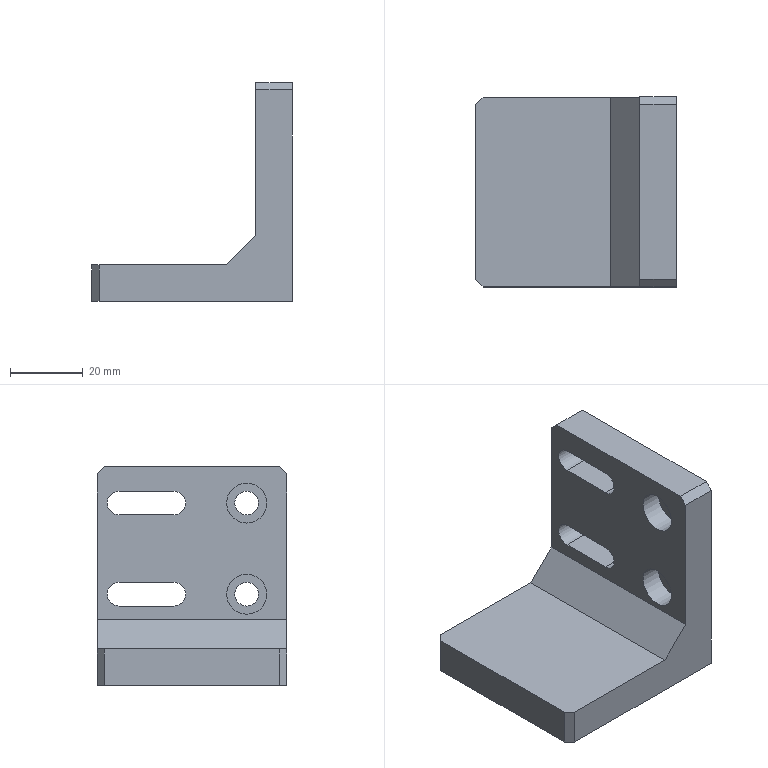Part | STEP file | Tube necking machine_id646_x_t | 1 solid | 27 faces | box 55 x 52 x 60 mm | volume 52164 mm3 | plane 19 | cylinder 8 | commonest cylinder face diameters 6.5 x6 11 x2